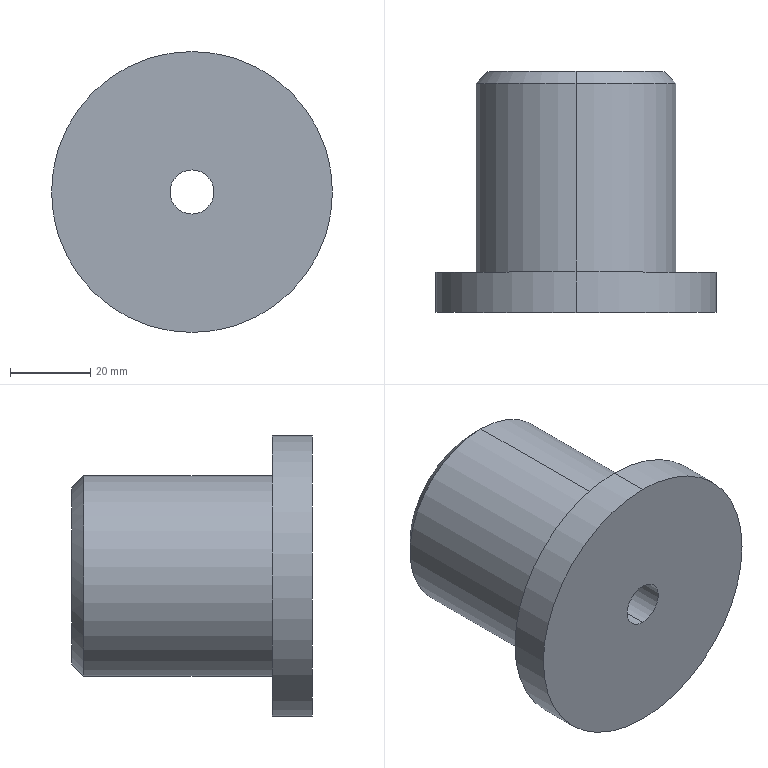Part | SolidWorks | features ICE 3, Chamfer 1, Extrusion 1 | 1 solid | 14 faces | box 70 x 60 x 70 mm | volume 128525 mm3 | cylinder 8 | plane 4 | cone 2 | commonest cylinder face diameters 11 x2 18 x2 50 x2 70 x2
STEP:
#1=CARTESIAN_POINT('',(0.,0.,-5.5));
#2=VERTEX_POINT('',#1);
#3=CARTESIAN_POINT('',(0.,0.,5.5));
#4=VERTEX_POINT('',#3);
#5=CARTESIAN_POINT('',(0.,0.,0.));
#6=DIRECTION('',(0.,1.,0.));
#7=DIRECTION('',(0.,0.,1.));
#8=AXIS2_PLACEMENT_3D('',#5,#6,#7);
#9=CIRCLE('',#8,5.5);
#10=EDGE_CURVE('',#2,#4,#9,.T.);
#11=ORIENTED_EDGE('',*,*,#10,.F.);
#12=CARTESIAN_POINT('',(0.,49.,-5.5));
#13=VERTEX_POINT('',#12);
#14=CARTESIAN_POINT('',(0.,-27.,-5.5));
#15=DIRECTION('',(0.,1.,0.));
#16=VECTOR('',#15,1000.);
#17=LINE('',#14,#16);
#18=EDGE_CURVE('',#2,#13,#17,.T.);
#19=ORIENTED_EDGE('',*,*,#18,.T.);
#20=CARTESIAN_POINT('',(0.,49.,5.5));
#21=VERTEX_POINT('',#20);
#22=CARTESIAN_POINT('',(0.,49.,0.));
#23=DIRECTION('',(0.,1.,0.));
#24=DIRECTION('',(0.,0.,1.));
#25=AXIS2_PLACEMENT_3D('',#22,#23,#24);
#26=CIRCLE('',#25,5.5);
#27=EDGE_CURVE('',#13,#21,#26,.T.);
#28=ORIENTED_EDGE('',*,*,#27,.T.);
#29=CARTESIAN_POINT('',(0.,-27.,5.5));
#30=DIRECTION('',(0.,1.,0.));
#31=VECTOR('',#30,1000.);
#32=LINE('',#29,#31);
#33=EDGE_CURVE('',#4,#21,#32,.T.);
#34=ORIENTED_EDGE('',*,*,#33,.F.);
#35=EDGE_LOOP('',(#11,#19,#28,#34));
#36=FACE_OUTER_BOUND('',#35,.T.);
#37=CARTESIAN_POINT('',(0.,-27.,0.));
#38=DIRECTION('',(0.,1.,0.));
#39=DIRECTION('',(0.,0.,1.));
#40=AXIS2_PLACEMENT_3D('',#37,#38,#39);
#41=CYLINDRICAL_SURFACE('',#40,5.5);
#42=ADVANCED_FACE('',(#36),#41,.F.);
#43=CARTESIAN_POINT('',(0.,49.,-9.));
#44=VERTEX_POINT('',#43);
#45=CARTESIAN_POINT('',(0.,49.,9.));
#46=VERTEX_POINT('',#45);
#47=CARTESIAN_POINT('',(0.,49.,0.));
#48=DIRECTION('',(0.,1.,0.));
#49=DIRECTION('',(0.,0.,1.));
#50=AXIS2_PLACEMENT_3D('',#47,#48,#49);
#51=CIRCLE('',#50,9.);
#52=EDGE_CURVE('',#44,#46,#51,.T.);
#53=ORIENTED_EDGE('',*,*,#52,.F.);
#54=CARTESIAN_POINT('',(0.,60.,-9.));
#55=VERTEX_POINT('',#54);
#56=CARTESIAN_POINT('',(0.,49.,-9.));
#57=DIRECTION('',(0.,1.,0.));
#58=VECTOR('',#57,1000.);
#59=LINE('',#56,#58);
#60=EDGE_CURVE('',#44,#55,#59,.T.);
#61=ORIENTED_EDGE('',*,*,#60,.T.);
#62=CARTESIAN_POINT('',(0.,60.,9.));
#63=VERTEX_POINT('',#62);
#64=CARTESIAN_POINT('',(0.,60.,0.));
#65=DIRECTION('',(0.,1.,0.));
#66=DIRECTION('',(0.,0.,1.));
#67=AXIS2_PLACEMENT_3D('',#64,#65,#66);
#68=CIRCLE('',#67,9.);
#69=EDGE_CURVE('',#55,#63,#68,.T.);
#70=ORIENTED_EDGE('',*,*,#69,.T.);
#71=CARTESIAN_POINT('',(0.,49.,9.));
#72=DIRECTION('',(0.,1.,0.));
#73=VECTOR('',#72,1000.);
#74=LINE('',#71,#73);
#75=EDGE_CURVE('',#46,#63,#74,.T.);
#76=ORIENTED_EDGE('',*,*,#75,.F.);
#77=EDGE_LOOP('',(#53,#61,#70,#76));
#78=FACE_OUTER_BOUND('',#77,.T.);
#79=CARTESIAN_POINT('',(0.,49.,0.));
#80=DIRECTION('',(0.,1.,0.));
#81=DIRECTION('',(0.,0.,1.));
#82=AXIS2_PLACEMENT_3D('',#79,#80,#81);
#83=CYLINDRICAL_SURFACE('',#82,9.);
#84=ADVANCED_FACE('',(#78),#83,.F.);
#85=CARTESIAN_POINT('',(0.,60.,22.));
#86=VERTEX_POINT('',#85);
#87=CARTESIAN_POINT('',(0.,60.,-22.));
#88=VERTEX_POINT('',#87);
#89=CARTESIAN_POINT('',(0.,60.,0.));
#90=DIRECTION('',(0.,1.,0.));
#91=DIRECTION('',(0.,0.,1.));
#92=AXIS2_PLACEMENT_3D('',#89,#90,#91);
#93=CIRCLE('',#92,22.);
#94=EDGE_CURVE('',#86,#88,#93,.T.);
#95=ORIENTED_EDGE('',*,*,#94,.F.);
#96=CARTESIAN_POINT('',(0.,57.,25.));
#97=VERTEX_POINT('',#96);
#98=CARTESIAN_POINT('',(0.,60.,22.));
#99=DIRECTION('',(0.,-0.7071,0.7071));
#100=VECTOR('',#99,1000.);
#101=LINE('',#98,#100);
#102=EDGE_CURVE('',#86,#97,#101,.T.);
#103=ORIENTED_EDGE('',*,*,#102,.T.);
#104=CARTESIAN_POINT('',(0.,57.,-25.));
#105=VERTEX_POINT('',#104);
#106=CARTESIAN_POINT('',(0.,57.,0.));
#107=DIRECTION('',(0.,-1.,0.));
#108=DIRECTION('',(0.,0.,1.));
#109=AXIS2_PLACEMENT_3D('',#106,#107,#108);
#110=CIRCLE('',#109,25.);
#111=EDGE_CURVE('',#105,#97,#110,.T.);
#112=ORIENTED_EDGE('',*,*,#111,.F.);
#113=CARTESIAN_POINT('',(0.,60.,-22.));
#114=DIRECTION('',(0.,-0.7071,-0.7071));
#115=VECTOR('',#114,1000.);
#116=LINE('',#113,#115);
#117=EDGE_CURVE('',#88,#105,#116,.T.);
#118=ORIENTED_EDGE('',*,*,#117,.F.);
#119=EDGE_LOOP('',(#95,#103,#112,#118));
#120=FACE_OUTER_BOUND('',#119,.T.);
#121=CARTESIAN_POINT('',(0.,60.,0.));
#122=DIRECTION('',(0.,-1.,0.));
#123=DIRECTION('',(0.,0.,-1.));
#124=AXIS2_PLACEMENT_3D('',#121,#122,#123);
#125=CONICAL_SURFACE('',#124,22.,0.7854);
#126=ADVANCED_FACE('',(#120),#125,.T.);
#127=ORIENTED_EDGE('',*,*,#111,.T.);
#128=CARTESIAN_POINT('',(0.,10.,25.));
#129=VERTEX_POINT('',#128);
#130=CARTESIAN_POINT('',(0.,60.,25.));
#131=DIRECTION('',(0.,-1.,0.));
#132=VECTOR('',#131,1000.);
#133=LINE('',#130,#132);
#134=EDGE_CURVE('',#97,#129,#133,.T.);
#135=ORIENTED_EDGE('',*,*,#134,.T.);
#136=CARTESIAN_POINT('',(0.,10.,-25.));
#137=VERTEX_POINT('',#136);
#138=CARTESIAN_POINT('',(0.,10.,0.));
#139=DIRECTION('',(0.,1.,0.));
#140=DIRECTION('',(0.,0.,1.));
#141=AXIS2_PLACEMENT_3D('',#138,#139,#140);
#142=CIRCLE('',#141,25.);
#143=EDGE_CURVE('',#129,#137,#142,.T.);
#144=ORIENTED_EDGE('',*,*,#143,.T.);
#145=CARTESIAN_POINT('',(0.,60.,-25.));
#146=DIRECTION('',(0.,-1.,0.));
#147=VECTOR('',#146,1000.);
#148=LINE('',#145,#147);
#149=EDGE_CURVE('',#105,#137,#148,.T.);
#150=ORIENTED_EDGE('',*,*,#149,.F.);
#151=EDGE_LOOP('',(#127,#135,#144,#150));
#152=FACE_OUTER_BOUND('',#151,.T.);
#153=CARTESIAN_POINT('',(0.,60.,0.));
#154=DIRECTION('',(0.,-1.,0.));
#155=DIRECTION('',(0.,0.,-1.));
#156=AXIS2_PLACEMENT_3D('',#153,#154,#155);
#157=CYLINDRICAL_SURFACE('',#156,25.);
#158=ADVANCED_FACE('',(#152),#157,.T.);
#159=CARTESIAN_POINT('',(0.,10.,35.));
#160=VERTEX_POINT('',#159);
#161=CARTESIAN_POINT('',(0.,10.,-35.));
#162=VERTEX_POINT('',#161);
#163=CARTESIAN_POINT('',(0.,10.,0.));
#164=DIRECTION('',(0.,1.,0.));
#165=DIRECTION('',(0.,0.,1.));
#166=AXIS2_PLACEMENT_3D('',#163,#164,#165);
#167=CIRCLE('',#166,35.);
#168=EDGE_CURVE('',#160,#162,#167,.T.);
#169=ORIENTED_EDGE('',*,*,#168,.F.);
#170=CARTESIAN_POINT('',(0.,0.,35.));
#171=VERTEX_POINT('',#170);
#172=CARTESIAN_POINT('',(0.,10.,35.));
#173=DIRECTION('',(0.,-1.,0.));
#174=VECTOR('',#173,1000.);
#175=LINE('',#172,#174);
#176=EDGE_CURVE('',#160,#171,#175,.T.);
#177=ORIENTED_EDGE('',*,*,#176,.T.);
#178=CARTESIAN_POINT('',(0.,0.,-35.));
#179=VERTEX_POINT('',#178);
#180=CARTESIAN_POINT('',(0.,0.,0.));
#181=DIRECTION('',(0.,1.,0.));
#182=DIRECTION('',(0.,0.,1.));
#183=AXIS2_PLACEMENT_3D('',#180,#181,#182);
#184=CIRCLE('',#183,35.);
#185=EDGE_CURVE('',#171,#179,#184,.T.);
#186=ORIENTED_EDGE('',*,*,#185,.T.);
#187=CARTESIAN_POINT('',(0.,10.,-35.));
#188=DIRECTION('',(0.,-1.,0.));
#189=VECTOR('',#188,1000.);
#190=LINE('',#187,#189);
#191=EDGE_CURVE('',#162,#179,#190,.T.);
#192=ORIENTED_EDGE('',*,*,#191,.F.);
#193=EDGE_LOOP('',(#169,#177,#186,#192));
#194=FACE_OUTER_BOUND('',#193,.T.);
#195=CARTESIAN_POINT('',(0.,10.,0.));
#196=DIRECTION('',(0.,-1.,0.));
#197=DIRECTION('',(0.,0.,-1.));
#198=AXIS2_PLACEMENT_3D('',#195,#196,#197);
#199=CYLINDRICAL_SURFACE('',#198,35.);
#200=ADVANCED_FACE('',(#194),#199,.T.);
#201=ORIENTED_EDGE('',*,*,#176,.F.);
#202=CARTESIAN_POINT('',(0.,10.,0.));
#203=DIRECTION('',(0.,1.,0.));
#204=DIRECTION('',(0.,0.,1.));
#205=AXIS2_PLACEMENT_3D('',#202,#203,#204);
#206=CIRCLE('',#205,35.);
#207=EDGE_CURVE('',#162,#160,#206,.T.);
#208=ORIENTED_EDGE('',*,*,#207,.F.);
#209=ORIENTED_EDGE('',*,*,#191,.T.);
#210=CARTESIAN_POINT('',(0.,0.,0.));
#211=DIRECTION('',(0.,1.,0.));
#212=DIRECTION('',(0.,0.,1.));
#213=AXIS2_PLACEMENT_3D('',#210,#211,#212);
#214=CIRCLE('',#213,35.);
#215=EDGE_CURVE('',#179,#171,#214,.T.);
#216=ORIENTED_EDGE('',*,*,#215,.T.);
#217=EDGE_LOOP('',(#201,#208,#209,#216));
#218=FACE_OUTER_BOUND('',#217,.T.);
#219=CARTESIAN_POINT('',(0.,10.,0.));
#220=DIRECTION('',(0.,-1.,0.));
#221=DIRECTION('',(0.,0.,-1.));
#222=AXIS2_PLACEMENT_3D('',#219,#220,#221);
#223=CYLINDRICAL_SURFACE('',#222,35.);
#224=ADVANCED_FACE('',(#218),#223,.T.);
#225=CARTESIAN_POINT('',(0.,10.,0.));
#226=DIRECTION('',(0.,1.,0.));
#227=DIRECTION('',(0.,0.,1.));
#228=AXIS2_PLACEMENT_3D('',#225,#226,#227);
#229=CIRCLE('',#228,25.);
#230=EDGE_CURVE('',#137,#129,#229,.T.);
#231=ORIENTED_EDGE('',*,*,#230,.F.);
#232=ORIENTED_EDGE('',*,*,#143,.F.);
#233=EDGE_LOOP('',(#231,#232));
#234=FACE_BOUND('',#233,.T.);
#235=ORIENTED_EDGE('',*,*,#207,.T.);
#236=ORIENTED_EDGE('',*,*,#168,.T.);
#237=EDGE_LOOP('',(#235,#236));
#238=FACE_OUTER_BOUND('',#237,.T.);
#239=CARTESIAN_POINT('',(0.,10.,0.));
#240=DIRECTION('',(0.,1.,0.));
#241=DIRECTION('',(0.,0.,1.));
#242=AXIS2_PLACEMENT_3D('',#239,#240,#241);
#243=PLANE('',#242);
#244=ADVANCED_FACE('',(#234,#238),#243,.T.);
#245=CARTESIAN_POINT('',(0.,0.,0.));
#246=DIRECTION('',(0.,1.,0.));
#247=DIRECTION('',(0.,0.,1.));
#248=AXIS2_PLACEMENT_3D('',#245,#246,#247);
#249=CIRCLE('',#248,5.5);
#250=EDGE_CURVE('',#4,#2,#249,.T.);
#251=ORIENTED_EDGE('',*,*,#250,.T.);
#252=ORIENTED_EDGE('',*,*,#10,.T.);
#253=EDGE_LOOP('',(#251,#252));
#254=FACE_BOUND('',#253,.T.);
#255=ORIENTED_EDGE('',*,*,#215,.F.);
#256=ORIENTED_EDGE('',*,*,#185,.F.);
#257=EDGE_LOOP('',(#255,#256));
#258=FACE_OUTER_BOUND('',#257,.T.);
#259=CARTESIAN_POINT('',(0.,0.,0.));
#260=DIRECTION('',(0.,1.,0.));
#261=DIRECTION('',(0.,0.,1.));
#262=AXIS2_PLACEMENT_3D('',#259,#260,#261);
#263=PLANE('',#262);
#264=ADVANCED_FACE('',(#254,#258),#263,.F.);
#265=ORIENTED_EDGE('',*,*,#134,.F.);
#266=CARTESIAN_POINT('',(0.,57.,0.));
#267=DIRECTION('',(0.,-1.,0.));
#268=DIRECTION('',(0.,0.,1.));
#269=AXIS2_PLACEMENT_3D('',#266,#267,#268);
#270=CIRCLE('',#269,25.);
#271=EDGE_CURVE('',#97,#105,#270,.T.);
#272=ORIENTED_EDGE('',*,*,#271,.T.);
#273=ORIENTED_EDGE('',*,*,#149,.T.);
#274=ORIENTED_EDGE('',*,*,#230,.T.);
#275=EDGE_LOOP('',(#265,#272,#273,#274));
#276=FACE_OUTER_BOUND('',#275,.T.);
#277=CARTESIAN_POINT('',(0.,60.,0.));
#278=DIRECTION('',(0.,-1.,0.));
#279=DIRECTION('',(0.,0.,-1.));
#280=AXIS2_PLACEMENT_3D('',#277,#278,#279);
#281=CYLINDRICAL_SURFACE('',#280,25.);
#282=ADVANCED_FACE('',(#276),#281,.T.);
#283=CARTESIAN_POINT('',(0.,60.,0.));
#284=DIRECTION('',(0.,1.,0.));
#285=DIRECTION('',(0.,0.,1.));
#286=AXIS2_PLACEMENT_3D('',#283,#284,#285);
#287=CIRCLE('',#286,9.);
#288=EDGE_CURVE('',#63,#55,#287,.T.);
#289=ORIENTED_EDGE('',*,*,#288,.F.);
#290=ORIENTED_EDGE('',*,*,#69,.F.);
#291=EDGE_LOOP('',(#289,#290));
#292=FACE_BOUND('',#291,.T.);
#293=CARTESIAN_POINT('',(0.,60.,0.));
#294=DIRECTION('',(0.,1.,0.));
#295=DIRECTION('',(0.,0.,1.));
#296=AXIS2_PLACEMENT_3D('',#293,#294,#295);
#297=CIRCLE('',#296,22.);
#298=EDGE_CURVE('',#88,#86,#297,.T.);
#299=ORIENTED_EDGE('',*,*,#298,.T.);
#300=ORIENTED_EDGE('',*,*,#94,.T.);
#301=EDGE_LOOP('',(#299,#300));
#302=FACE_OUTER_BOUND('',#301,.T.);
#303=CARTESIAN_POINT('',(0.,60.,0.));
#304=DIRECTION('',(0.,1.,0.));
#305=DIRECTION('',(0.,0.,1.));
#306=AXIS2_PLACEMENT_3D('',#303,#304,#305);
#307=PLANE('',#306);
#308=ADVANCED_FACE('',(#292,#302),#307,.T.);
#309=ORIENTED_EDGE('',*,*,#102,.F.);
#310=ORIENTED_EDGE('',*,*,#298,.F.);
#311=ORIENTED_EDGE('',*,*,#117,.T.);
#312=ORIENTED_EDGE('',*,*,#271,.F.);
#313=EDGE_LOOP('',(#309,#310,#311,#312));
#314=FACE_OUTER_BOUND('',#313,.T.);
#315=CARTESIAN_POINT('',(0.,60.,0.));
#316=DIRECTION('',(0.,-1.,0.));
#317=DIRECTION('',(0.,0.,-1.));
#318=AXIS2_PLACEMENT_3D('',#315,#316,#317);
#319=CONICAL_SURFACE('',#318,22.,0.7854);
#320=ADVANCED_FACE('',(#314),#319,.T.);
#321=ORIENTED_EDGE('',*,*,#60,.F.);
#322=CARTESIAN_POINT('',(0.,49.,0.));
#323=DIRECTION('',(0.,1.,0.));
#324=DIRECTION('',(0.,0.,1.));
#325=AXIS2_PLACEMENT_3D('',#322,#323,#324);
#326=CIRCLE('',#325,9.);
#327=EDGE_CURVE('',#46,#44,#326,.T.);
#328=ORIENTED_EDGE('',*,*,#327,.F.);
#329=ORIENTED_EDGE('',*,*,#75,.T.);
#330=ORIENTED_EDGE('',*,*,#288,.T.);
#331=EDGE_LOOP('',(#321,#328,#329,#330));
#332=FACE_OUTER_BOUND('',#331,.T.);
#333=CARTESIAN_POINT('',(0.,49.,0.));
#334=DIRECTION('',(0.,1.,0.));
#335=DIRECTION('',(0.,0.,1.));
#336=AXIS2_PLACEMENT_3D('',#333,#334,#335);
#337=CYLINDRICAL_SURFACE('',#336,9.);
#338=ADVANCED_FACE('',(#332),#337,.F.);
#339=CARTESIAN_POINT('',(0.,49.,0.));
#340=DIRECTION('',(0.,1.,0.));
#341=DIRECTION('',(0.,0.,1.));
#342=AXIS2_PLACEMENT_3D('',#339,#340,#341);
#343=CIRCLE('',#342,5.5);
#344=EDGE_CURVE('',#21,#13,#343,.T.);
#345=ORIENTED_EDGE('',*,*,#344,.F.);
#346=ORIENTED_EDGE('',*,*,#27,.F.);
#347=EDGE_LOOP('',(#345,#346));
#348=FACE_BOUND('',#347,.T.);
#349=ORIENTED_EDGE('',*,*,#327,.T.);
#350=ORIENTED_EDGE('',*,*,#52,.T.);
#351=EDGE_LOOP('',(#349,#350));
#352=FACE_OUTER_BOUND('',#351,.T.);
#353=CARTESIAN_POINT('',(0.,49.,0.));
#354=DIRECTION('',(0.,1.,0.));
#355=DIRECTION('',(0.,0.,1.));
#356=AXIS2_PLACEMENT_3D('',#353,#354,#355);
#357=PLANE('',#356);
#358=ADVANCED_FACE('',(#348,#352),#357,.T.);
#359=ORIENTED_EDGE('',*,*,#18,.F.);
#360=ORIENTED_EDGE('',*,*,#250,.F.);
#361=ORIENTED_EDGE('',*,*,#33,.T.);
#362=ORIENTED_EDGE('',*,*,#344,.T.);
#363=EDGE_LOOP('',(#359,#360,#361,#362));
#364=FACE_OUTER_BOUND('',#363,.T.);
#365=CARTESIAN_POINT('',(0.,-27.,0.));
#366=DIRECTION('',(0.,1.,0.));
#367=DIRECTION('',(0.,0.,1.));
#368=AXIS2_PLACEMENT_3D('',#365,#366,#367);
#369=CYLINDRICAL_SURFACE('',#368,5.5);
#370=ADVANCED_FACE('',(#364),#369,.F.);
#371=CLOSED_SHELL('',(#42,#84,#126,#158,#200,#224,#244,#264,#282,#308,#320,#338,#358,#370));
#372=MANIFOLD_SOLID_BREP('',#371);
#373=CARTESIAN_POINT('',(0.,0.,0.));
#374=DIRECTION('',(0.,0.,1.));
#375=DIRECTION('',(1.,0.,0.));
#376=AXIS2_PLACEMENT_3D('',#373,#374,#375);
#377=(LENGTH_UNIT()NAMED_UNIT(*)SI_UNIT(.MILLI.,.METRE.));
#378=UNCERTAINTY_MEASURE_WITH_UNIT(LENGTH_MEASURE(0.00001),#377,'','');
#379=(NAMED_UNIT(*)PLANE_ANGLE_UNIT()SI_UNIT($,.RADIAN.));
#380=(NAMED_UNIT(*)SI_UNIT($,.STERADIAN.)SOLID_ANGLE_UNIT());
#381=(GEOMETRIC_REPRESENTATION_CONTEXT(3)GLOBAL_UNCERTAINTY_ASSIGNED_CONTEXT((#378))GLOBAL_UNIT_ASSIGNED_CONTEXT((#377,#379,#380))REPRESENTATION_CONTEXT('',''));
#382=ADVANCED_BREP_SHAPE_REPRESENTATION('',(#372,#376),#381);